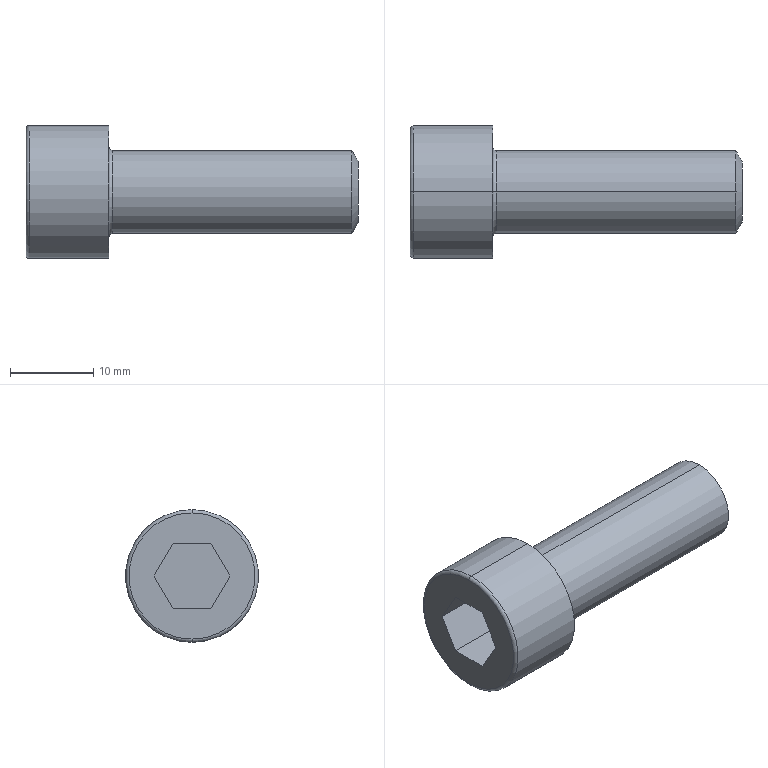Part | SolidWorks | features BaseBody 1 | 1 solid | 20 faces | box 40 x 16 x 16 mm | volume 4026 mm3 | plane 10 | torus 4 | cylinder 4 | cone 2 | commonest cylinder face diameters 10 x2 16 x2
STEP:
#1=CARTESIAN_POINT('',(40.,0.,3.701));
#2=VERTEX_POINT('',#1);
#3=CARTESIAN_POINT('',(40.,0.,-3.701));
#4=VERTEX_POINT('',#3);
#5=CARTESIAN_POINT('',(40.,0.,0.));
#6=DIRECTION('',(-1.,0.,0.));
#7=DIRECTION('',(0.,0.,1.));
#8=AXIS2_PLACEMENT_3D('',#5,#6,#7);
#9=CIRCLE('',#8,3.701);
#10=EDGE_CURVE('',#2,#4,#9,.T.);
#11=ORIENTED_EDGE('',*,*,#10,.T.);
#12=CARTESIAN_POINT('',(39.25,0.,-5.));
#13=VERTEX_POINT('',#12);
#14=CARTESIAN_POINT('',(39.25,0.,-5.));
#15=DIRECTION('',(-0.5,0.,-0.866));
#16=VECTOR('',#15,1000.);
#17=LINE('',#14,#16);
#18=EDGE_CURVE('',#4,#13,#17,.T.);
#19=ORIENTED_EDGE('',*,*,#18,.T.);
#20=CARTESIAN_POINT('',(39.25,0.,5.));
#21=VERTEX_POINT('',#20);
#22=CARTESIAN_POINT('',(39.25,0.,0.));
#23=DIRECTION('',(-1.,0.,0.));
#24=DIRECTION('',(0.,0.,1.));
#25=AXIS2_PLACEMENT_3D('',#22,#23,#24);
#26=CIRCLE('',#25,5.);
#27=EDGE_CURVE('',#21,#13,#26,.T.);
#28=ORIENTED_EDGE('',*,*,#27,.F.);
#29=CARTESIAN_POINT('',(39.25,0.,5.));
#30=DIRECTION('',(-0.5,0.,0.866));
#31=VECTOR('',#30,1000.);
#32=LINE('',#29,#31);
#33=EDGE_CURVE('',#2,#21,#32,.T.);
#34=ORIENTED_EDGE('',*,*,#33,.F.);
#35=EDGE_LOOP('',(#11,#19,#28,#34));
#36=FACE_OUTER_BOUND('',#35,.T.);
#37=CARTESIAN_POINT('',(39.25,0.,0.));
#38=DIRECTION('',(-1.,0.,0.));
#39=DIRECTION('',(0.,0.,1.));
#40=AXIS2_PLACEMENT_3D('',#37,#38,#39);
#41=CONICAL_SURFACE('',#40,5.,1.047);
#42=ADVANCED_FACE('',(#36),#41,.T.);
#43=CARTESIAN_POINT('',(0.4,0.,-8.));
#44=VERTEX_POINT('',#43);
#45=CARTESIAN_POINT('',(0.4,0.,8.));
#46=VERTEX_POINT('',#45);
#47=CARTESIAN_POINT('',(0.4,0.,0.));
#48=DIRECTION('',(1.,0.,0.));
#49=DIRECTION('',(0.,0.,1.));
#50=AXIS2_PLACEMENT_3D('',#47,#48,#49);
#51=CIRCLE('',#50,8.);
#52=EDGE_CURVE('',#44,#46,#51,.T.);
#53=ORIENTED_EDGE('',*,*,#52,.F.);
#54=CARTESIAN_POINT('',(0.,0.,-7.6));
#55=VERTEX_POINT('',#54);
#56=CARTESIAN_POINT('',(0.4,0.,-7.6));
#57=DIRECTION('',(0.,1.,0.));
#58=DIRECTION('',(0.,0.,1.));
#59=AXIS2_PLACEMENT_3D('',#56,#57,#58);
#60=CIRCLE('',#59,0.4);
#61=EDGE_CURVE('',#44,#55,#60,.T.);
#62=ORIENTED_EDGE('',*,*,#61,.T.);
#63=CARTESIAN_POINT('',(0.,0.,7.6));
#64=VERTEX_POINT('',#63);
#65=CARTESIAN_POINT('',(0.,0.,0.));
#66=DIRECTION('',(-1.,0.,0.));
#67=DIRECTION('',(0.,0.,1.));
#68=AXIS2_PLACEMENT_3D('',#65,#66,#67);
#69=CIRCLE('',#68,7.6);
#70=EDGE_CURVE('',#64,#55,#69,.T.);
#71=ORIENTED_EDGE('',*,*,#70,.F.);
#72=CARTESIAN_POINT('',(0.4,0.,7.6));
#73=DIRECTION('',(0.,-1.,0.));
#74=DIRECTION('',(0.,0.,-1.));
#75=AXIS2_PLACEMENT_3D('',#72,#73,#74);
#76=CIRCLE('',#75,0.4);
#77=EDGE_CURVE('',#46,#64,#76,.T.);
#78=ORIENTED_EDGE('',*,*,#77,.F.);
#79=EDGE_LOOP('',(#53,#62,#71,#78));
#80=FACE_OUTER_BOUND('',#79,.T.);
#81=CARTESIAN_POINT('',(0.4,0.,0.));
#82=DIRECTION('',(-1.,0.,0.));
#83=DIRECTION('',(0.,0.,1.));
#84=AXIS2_PLACEMENT_3D('',#81,#82,#83);
#85=TOROIDAL_SURFACE('',#84,7.6,0.4);
#86=ADVANCED_FACE('',(#80),#85,.T.);
#87=CARTESIAN_POINT('',(10.4,0.,5.));
#88=VERTEX_POINT('',#87);
#89=CARTESIAN_POINT('',(10.4,0.,-5.));
#90=VERTEX_POINT('',#89);
#91=CARTESIAN_POINT('',(10.4,0.,0.));
#92=DIRECTION('',(1.,0.,0.));
#93=DIRECTION('',(0.,0.,-1.));
#94=AXIS2_PLACEMENT_3D('',#91,#92,#93);
#95=CIRCLE('',#94,5.);
#96=EDGE_CURVE('',#88,#90,#95,.T.);
#97=ORIENTED_EDGE('',*,*,#96,.F.);
#98=CARTESIAN_POINT('',(10.,0.,5.4));
#99=VERTEX_POINT('',#98);
#100=CARTESIAN_POINT('',(10.4,0.,5.4));
#101=DIRECTION('',(0.,1.,0.));
#102=DIRECTION('',(0.,0.,1.));
#103=AXIS2_PLACEMENT_3D('',#100,#101,#102);
#104=CIRCLE('',#103,0.4);
#105=EDGE_CURVE('',#88,#99,#104,.T.);
#106=ORIENTED_EDGE('',*,*,#105,.T.);
#107=CARTESIAN_POINT('',(10.,0.,-5.4));
#108=VERTEX_POINT('',#107);
#109=CARTESIAN_POINT('',(10.,0.,0.));
#110=DIRECTION('',(1.,0.,0.));
#111=DIRECTION('',(0.,0.,-1.));
#112=AXIS2_PLACEMENT_3D('',#109,#110,#111);
#113=CIRCLE('',#112,5.4);
#114=EDGE_CURVE('',#99,#108,#113,.T.);
#115=ORIENTED_EDGE('',*,*,#114,.T.);
#116=CARTESIAN_POINT('',(10.4,0.,-5.4));
#117=DIRECTION('',(0.,-1.,0.));
#118=DIRECTION('',(0.,0.,-1.));
#119=AXIS2_PLACEMENT_3D('',#116,#117,#118);
#120=CIRCLE('',#119,0.4);
#121=EDGE_CURVE('',#90,#108,#120,.T.);
#122=ORIENTED_EDGE('',*,*,#121,.F.);
#123=EDGE_LOOP('',(#97,#106,#115,#122));
#124=FACE_OUTER_BOUND('',#123,.T.);
#125=CARTESIAN_POINT('',(10.4,0.,0.));
#126=DIRECTION('',(1.,0.,0.));
#127=DIRECTION('',(0.,0.,-1.));
#128=AXIS2_PLACEMENT_3D('',#125,#126,#127);
#129=TOROIDAL_SURFACE('',#128,5.4,0.4);
#130=ADVANCED_FACE('',(#124),#129,.F.);
#131=ORIENTED_EDGE('',*,*,#52,.T.);
#132=CARTESIAN_POINT('',(10.,0.,8.));
#133=VERTEX_POINT('',#132);
#134=CARTESIAN_POINT('',(0.,0.,8.));
#135=DIRECTION('',(1.,0.,0.));
#136=VECTOR('',#135,1000.);
#137=LINE('',#134,#136);
#138=EDGE_CURVE('',#46,#133,#137,.T.);
#139=ORIENTED_EDGE('',*,*,#138,.T.);
#140=CARTESIAN_POINT('',(10.,0.,-8.));
#141=VERTEX_POINT('',#140);
#142=CARTESIAN_POINT('',(10.,0.,0.));
#143=DIRECTION('',(1.,0.,0.));
#144=DIRECTION('',(0.,0.,-1.));
#145=AXIS2_PLACEMENT_3D('',#142,#143,#144);
#146=CIRCLE('',#145,8.);
#147=EDGE_CURVE('',#141,#133,#146,.T.);
#148=ORIENTED_EDGE('',*,*,#147,.F.);
#149=CARTESIAN_POINT('',(0.,0.,-8.));
#150=DIRECTION('',(1.,0.,0.));
#151=VECTOR('',#150,1000.);
#152=LINE('',#149,#151);
#153=EDGE_CURVE('',#44,#141,#152,.T.);
#154=ORIENTED_EDGE('',*,*,#153,.F.);
#155=EDGE_LOOP('',(#131,#139,#148,#154));
#156=FACE_OUTER_BOUND('',#155,.T.);
#157=CARTESIAN_POINT('',(0.,0.,0.));
#158=DIRECTION('',(1.,0.,0.));
#159=DIRECTION('',(0.,0.,-1.));
#160=AXIS2_PLACEMENT_3D('',#157,#158,#159);
#161=CYLINDRICAL_SURFACE('',#160,8.);
#162=ADVANCED_FACE('',(#156),#161,.T.);
#163=CARTESIAN_POINT('',(10.4,0.,0.));
#164=DIRECTION('',(1.,0.,0.));
#165=DIRECTION('',(0.,0.,-1.));
#166=AXIS2_PLACEMENT_3D('',#163,#164,#165);
#167=CIRCLE('',#166,5.);
#168=EDGE_CURVE('',#90,#88,#167,.T.);
#169=ORIENTED_EDGE('',*,*,#168,.T.);
#170=CARTESIAN_POINT('',(0.,0.,5.));
#171=DIRECTION('',(1.,0.,0.));
#172=VECTOR('',#171,1000.);
#173=LINE('',#170,#172);
#174=EDGE_CURVE('',#88,#21,#173,.T.);
#175=ORIENTED_EDGE('',*,*,#174,.T.);
#176=ORIENTED_EDGE('',*,*,#27,.T.);
#177=CARTESIAN_POINT('',(0.,0.,-5.));
#178=DIRECTION('',(1.,0.,0.));
#179=VECTOR('',#178,1000.);
#180=LINE('',#177,#179);
#181=EDGE_CURVE('',#90,#13,#180,.T.);
#182=ORIENTED_EDGE('',*,*,#181,.F.);
#183=EDGE_LOOP('',(#169,#175,#176,#182));
#184=FACE_OUTER_BOUND('',#183,.T.);
#185=CARTESIAN_POINT('',(0.,0.,0.));
#186=DIRECTION('',(1.,0.,0.));
#187=DIRECTION('',(0.,0.,-1.));
#188=AXIS2_PLACEMENT_3D('',#185,#186,#187);
#189=CYLINDRICAL_SURFACE('',#188,5.);
#190=ADVANCED_FACE('',(#184),#189,.T.);
#191=ORIENTED_EDGE('',*,*,#174,.F.);
#192=ORIENTED_EDGE('',*,*,#96,.T.);
#193=ORIENTED_EDGE('',*,*,#181,.T.);
#194=CARTESIAN_POINT('',(39.25,0.,0.));
#195=DIRECTION('',(-1.,0.,0.));
#196=DIRECTION('',(0.,0.,1.));
#197=AXIS2_PLACEMENT_3D('',#194,#195,#196);
#198=CIRCLE('',#197,5.);
#199=EDGE_CURVE('',#13,#21,#198,.T.);
#200=ORIENTED_EDGE('',*,*,#199,.T.);
#201=EDGE_LOOP('',(#191,#192,#193,#200));
#202=FACE_OUTER_BOUND('',#201,.T.);
#203=CARTESIAN_POINT('',(0.,0.,0.));
#204=DIRECTION('',(1.,0.,0.));
#205=DIRECTION('',(0.,0.,-1.));
#206=AXIS2_PLACEMENT_3D('',#203,#204,#205);
#207=CYLINDRICAL_SURFACE('',#206,5.);
#208=ADVANCED_FACE('',(#202),#207,.T.);
#209=ORIENTED_EDGE('',*,*,#70,.T.);
#210=CARTESIAN_POINT('',(0.,0.,0.));
#211=DIRECTION('',(-1.,0.,0.));
#212=DIRECTION('',(0.,0.,1.));
#213=AXIS2_PLACEMENT_3D('',#210,#211,#212);
#214=CIRCLE('',#213,7.6);
#215=EDGE_CURVE('',#55,#64,#214,.T.);
#216=ORIENTED_EDGE('',*,*,#215,.T.);
#217=EDGE_LOOP('',(#209,#216));
#218=FACE_OUTER_BOUND('',#217,.T.);
#219=CARTESIAN_POINT('',(0.,-4.575,0.));
#220=VERTEX_POINT('',#219);
#221=CARTESIAN_POINT('',(0.,-2.288,3.962));
#222=VERTEX_POINT('',#221);
#223=CARTESIAN_POINT('',(0.,-4.575,0.));
#224=DIRECTION('',(0.,0.5,0.866));
#225=VECTOR('',#224,1000.);
#226=LINE('',#223,#225);
#227=EDGE_CURVE('',#220,#222,#226,.T.);
#228=ORIENTED_EDGE('',*,*,#227,.F.);
#229=CARTESIAN_POINT('',(0.,-2.288,-3.962));
#230=VERTEX_POINT('',#229);
#231=CARTESIAN_POINT('',(0.,-2.288,-3.962));
#232=DIRECTION('',(0.,-0.5,0.866));
#233=VECTOR('',#232,1000.);
#234=LINE('',#231,#233);
#235=EDGE_CURVE('',#230,#220,#234,.T.);
#236=ORIENTED_EDGE('',*,*,#235,.F.);
#237=CARTESIAN_POINT('',(0.,2.288,-3.962));
#238=VERTEX_POINT('',#237);
#239=CARTESIAN_POINT('',(0.,2.288,-3.962));
#240=DIRECTION('',(0.,-1.,0.));
#241=VECTOR('',#240,1000.);
#242=LINE('',#239,#241);
#243=EDGE_CURVE('',#238,#230,#242,.T.);
#244=ORIENTED_EDGE('',*,*,#243,.F.);
#245=CARTESIAN_POINT('',(0.,4.575,0.));
#246=VERTEX_POINT('',#245);
#247=CARTESIAN_POINT('',(0.,4.575,0.));
#248=DIRECTION('',(0.,-0.5,-0.866));
#249=VECTOR('',#248,1000.);
#250=LINE('',#247,#249);
#251=EDGE_CURVE('',#246,#238,#250,.T.);
#252=ORIENTED_EDGE('',*,*,#251,.F.);
#253=CARTESIAN_POINT('',(0.,2.288,3.962));
#254=VERTEX_POINT('',#253);
#255=CARTESIAN_POINT('',(0.,2.288,3.962));
#256=DIRECTION('',(0.,0.5,-0.866));
#257=VECTOR('',#256,1000.);
#258=LINE('',#255,#257);
#259=EDGE_CURVE('',#254,#246,#258,.T.);
#260=ORIENTED_EDGE('',*,*,#259,.F.);
#261=CARTESIAN_POINT('',(0.,-2.288,3.962));
#262=DIRECTION('',(0.,1.,0.));
#263=VECTOR('',#262,1000.);
#264=LINE('',#261,#263);
#265=EDGE_CURVE('',#222,#254,#264,.T.);
#266=ORIENTED_EDGE('',*,*,#265,.F.);
#267=EDGE_LOOP('',(#228,#236,#244,#252,#260,#266));
#268=FACE_BOUND('',#267,.T.);
#269=CARTESIAN_POINT('',(0.,0.,0.));
#270=DIRECTION('',(-1.,0.,0.));
#271=DIRECTION('',(0.,0.,1.));
#272=AXIS2_PLACEMENT_3D('',#269,#270,#271);
#273=PLANE('',#272);
#274=ADVANCED_FACE('',(#218,#268),#273,.T.);
#275=ORIENTED_EDGE('',*,*,#138,.F.);
#276=CARTESIAN_POINT('',(0.4,0.,0.));
#277=DIRECTION('',(1.,0.,0.));
#278=DIRECTION('',(0.,0.,1.));
#279=AXIS2_PLACEMENT_3D('',#276,#277,#278);
#280=CIRCLE('',#279,8.);
#281=EDGE_CURVE('',#46,#44,#280,.T.);
#282=ORIENTED_EDGE('',*,*,#281,.T.);
#283=ORIENTED_EDGE('',*,*,#153,.T.);
#284=CARTESIAN_POINT('',(10.,0.,0.));
#285=DIRECTION('',(1.,0.,0.));
#286=DIRECTION('',(0.,0.,-1.));
#287=AXIS2_PLACEMENT_3D('',#284,#285,#286);
#288=CIRCLE('',#287,8.);
#289=EDGE_CURVE('',#133,#141,#288,.T.);
#290=ORIENTED_EDGE('',*,*,#289,.F.);
#291=EDGE_LOOP('',(#275,#282,#283,#290));
#292=FACE_OUTER_BOUND('',#291,.T.);
#293=CARTESIAN_POINT('',(0.,0.,0.));
#294=DIRECTION('',(1.,0.,0.));
#295=DIRECTION('',(0.,0.,-1.));
#296=AXIS2_PLACEMENT_3D('',#293,#294,#295);
#297=CYLINDRICAL_SURFACE('',#296,8.);
#298=ADVANCED_FACE('',(#292),#297,.T.);
#299=ORIENTED_EDGE('',*,*,#147,.T.);
#300=ORIENTED_EDGE('',*,*,#289,.T.);
#301=EDGE_LOOP('',(#299,#300));
#302=FACE_OUTER_BOUND('',#301,.T.);
#303=CARTESIAN_POINT('',(10.,0.,0.));
#304=DIRECTION('',(1.,0.,0.));
#305=DIRECTION('',(0.,0.,-1.));
#306=AXIS2_PLACEMENT_3D('',#303,#304,#305);
#307=CIRCLE('',#306,5.4);
#308=EDGE_CURVE('',#108,#99,#307,.T.);
#309=ORIENTED_EDGE('',*,*,#308,.F.);
#310=ORIENTED_EDGE('',*,*,#114,.F.);
#311=EDGE_LOOP('',(#309,#310));
#312=FACE_BOUND('',#311,.T.);
#313=CARTESIAN_POINT('',(10.,8.,0.));
#314=DIRECTION('',(1.,0.,0.));
#315=DIRECTION('',(0.,0.,-1.));
#316=AXIS2_PLACEMENT_3D('',#313,#314,#315);
#317=PLANE('',#316);
#318=ADVANCED_FACE('',(#302,#312),#317,.T.);
#319=ORIENTED_EDGE('',*,*,#105,.F.);
#320=ORIENTED_EDGE('',*,*,#168,.F.);
#321=ORIENTED_EDGE('',*,*,#121,.T.);
#322=ORIENTED_EDGE('',*,*,#308,.T.);
#323=EDGE_LOOP('',(#319,#320,#321,#322));
#324=FACE_OUTER_BOUND('',#323,.T.);
#325=CARTESIAN_POINT('',(10.4,0.,0.));
#326=DIRECTION('',(1.,0.,0.));
#327=DIRECTION('',(0.,0.,-1.));
#328=AXIS2_PLACEMENT_3D('',#325,#326,#327);
#329=TOROIDAL_SURFACE('',#328,5.4,0.4);
#330=ADVANCED_FACE('',(#324),#329,.F.);
#331=ORIENTED_EDGE('',*,*,#227,.T.);
#332=CARTESIAN_POINT('',(6.,-2.288,3.962));
#333=VERTEX_POINT('',#332);
#334=CARTESIAN_POINT('',(6.,-2.288,3.962));
#335=DIRECTION('',(-1.,0.,0.));
#336=VECTOR('',#335,1000.);
#337=LINE('',#334,#336);
#338=EDGE_CURVE('',#333,#222,#337,.T.);
#339=ORIENTED_EDGE('',*,*,#338,.F.);
#340=CARTESIAN_POINT('',(6.,-4.575,0.));
#341=VERTEX_POINT('',#340);
#342=CARTESIAN_POINT('',(6.,-4.575,0.));
#343=DIRECTION('',(0.,0.5,0.866));
#344=VECTOR('',#343,1000.);
#345=LINE('',#342,#344);
#346=EDGE_CURVE('',#341,#333,#345,.T.);
#347=ORIENTED_EDGE('',*,*,#346,.F.);
#348=CARTESIAN_POINT('',(6.,-4.575,0.));
#349=DIRECTION('',(-1.,0.,0.));
#350=VECTOR('',#349,1000.);
#351=LINE('',#348,#350);
#352=EDGE_CURVE('',#341,#220,#351,.T.);
#353=ORIENTED_EDGE('',*,*,#352,.T.);
#354=EDGE_LOOP('',(#331,#339,#347,#353));
#355=FACE_OUTER_BOUND('',#354,.T.);
#356=CARTESIAN_POINT('',(6.,-4.575,0.));
#357=DIRECTION('',(0.,-0.866,0.5));
#358=DIRECTION('',(0.,-0.5,-0.866));
#359=AXIS2_PLACEMENT_3D('',#356,#357,#358);
#360=PLANE('',#359);
#361=ADVANCED_FACE('',(#355),#360,.F.);
#362=ORIENTED_EDGE('',*,*,#235,.T.);
#363=ORIENTED_EDGE('',*,*,#352,.F.);
#364=CARTESIAN_POINT('',(6.,-2.288,-3.962));
#365=VERTEX_POINT('',#364);
#366=CARTESIAN_POINT('',(6.,-2.288,-3.962));
#367=DIRECTION('',(0.,-0.5,0.866));
#368=VECTOR('',#367,1000.);
#369=LINE('',#366,#368);
#370=EDGE_CURVE('',#365,#341,#369,.T.);
#371=ORIENTED_EDGE('',*,*,#370,.F.);
#372=CARTESIAN_POINT('',(6.,-2.288,-3.962));
#373=DIRECTION('',(-1.,0.,0.));
#374=VECTOR('',#373,1000.);
#375=LINE('',#372,#374);
#376=EDGE_CURVE('',#365,#230,#375,.T.);
#377=ORIENTED_EDGE('',*,*,#376,.T.);
#378=EDGE_LOOP('',(#362,#363,#371,#377));
#379=FACE_OUTER_BOUND('',#378,.T.);
#380=CARTESIAN_POINT('',(6.,-2.288,-3.962));
#381=DIRECTION('',(0.,-0.866,-0.5));
#382=DIRECTION('',(0.,0.5,-0.866));
#383=AXIS2_PLACEMENT_3D('',#380,#381,#382);
#384=PLANE('',#383);
#385=ADVANCED_FACE('',(#379),#384,.F.);
#386=ORIENTED_EDGE('',*,*,#243,.T.);
#387=ORIENTED_EDGE('',*,*,#376,.F.);
#388=CARTESIAN_POINT('',(6.,2.288,-3.962));
#389=VERTEX_POINT('',#388);
#390=CARTESIAN_POINT('',(6.,2.288,-3.962));
#391=DIRECTION('',(0.,-1.,0.));
#392=VECTOR('',#391,1000.);
#393=LINE('',#390,#392);
#394=EDGE_CURVE('',#389,#365,#393,.T.);
#395=ORIENTED_EDGE('',*,*,#394,.F.);
#396=CARTESIAN_POINT('',(6.,2.288,-3.962));
#397=DIRECTION('',(-1.,0.,0.));
#398=VECTOR('',#397,1000.);
#399=LINE('',#396,#398);
#400=EDGE_CURVE('',#389,#238,#399,.T.);
#401=ORIENTED_EDGE('',*,*,#400,.T.);
#402=EDGE_LOOP('',(#386,#387,#395,#401));
#403=FACE_OUTER_BOUND('',#402,.T.);
#404=CARTESIAN_POINT('',(6.,2.288,-3.962));
#405=DIRECTION('',(0.,0.,-1.));
#406=DIRECTION('',(0.,1.,0.));
#407=AXIS2_PLACEMENT_3D('',#404,#405,#406);
#408=PLANE('',#407);
#409=ADVANCED_FACE('',(#403),#408,.F.);
#410=ORIENTED_EDGE('',*,*,#251,.T.);
#411=ORIENTED_EDGE('',*,*,#400,.F.);
#412=CARTESIAN_POINT('',(6.,4.575,0.));
#413=VERTEX_POINT('',#412);
#414=CARTESIAN_POINT('',(6.,4.575,0.));
#415=DIRECTION('',(0.,-0.5,-0.866));
#416=VECTOR('',#415,1000.);
#417=LINE('',#414,#416);
#418=EDGE_CURVE('',#413,#389,#417,.T.);
#419=ORIENTED_EDGE('',*,*,#418,.F.);
#420=CARTESIAN_POINT('',(6.,4.575,0.));
#421=DIRECTION('',(-1.,0.,0.));
#422=VECTOR('',#421,1000.);
#423=LINE('',#420,#422);
#424=EDGE_CURVE('',#413,#246,#423,.T.);
#425=ORIENTED_EDGE('',*,*,#424,.T.);
#426=EDGE_LOOP('',(#410,#411,#419,#425));
#427=FACE_OUTER_BOUND('',#426,.T.);
#428=CARTESIAN_POINT('',(6.,4.575,0.));
#429=DIRECTION('',(0.,0.866,-0.5));
#430=DIRECTION('',(0.,0.5,0.866));
#431=AXIS2_PLACEMENT_3D('',#428,#429,#430);
#432=PLANE('',#431);
#433=ADVANCED_FACE('',(#427),#432,.F.);
#434=ORIENTED_EDGE('',*,*,#259,.T.);
#435=ORIENTED_EDGE('',*,*,#424,.F.);
#436=CARTESIAN_POINT('',(6.,2.288,3.962));
#437=VERTEX_POINT('',#436);
#438=CARTESIAN_POINT('',(6.,2.288,3.962));
#439=DIRECTION('',(0.,0.5,-0.866));
#440=VECTOR('',#439,1000.);
#441=LINE('',#438,#440);
#442=EDGE_CURVE('',#437,#413,#441,.T.);
#443=ORIENTED_EDGE('',*,*,#442,.F.);
#444=CARTESIAN_POINT('',(6.,2.288,3.962));
#445=DIRECTION('',(-1.,0.,0.));
#446=VECTOR('',#445,1000.);
#447=LINE('',#444,#446);
#448=EDGE_CURVE('',#437,#254,#447,.T.);
#449=ORIENTED_EDGE('',*,*,#448,.T.);
#450=EDGE_LOOP('',(#434,#435,#443,#449));
#451=FACE_OUTER_BOUND('',#450,.T.);
#452=CARTESIAN_POINT('',(6.,2.288,3.962));
#453=DIRECTION('',(0.,0.866,0.5));
#454=DIRECTION('',(0.,-0.5,0.866));
#455=AXIS2_PLACEMENT_3D('',#452,#453,#454);
#456=PLANE('',#455);
#457=ADVANCED_FACE('',(#451),#456,.F.);
#458=ORIENTED_EDGE('',*,*,#265,.T.);
#459=ORIENTED_EDGE('',*,*,#448,.F.);
#460=CARTESIAN_POINT('',(6.,-2.288,3.962));
#461=DIRECTION('',(0.,1.,0.));
#462=VECTOR('',#461,1000.);
#463=LINE('',#460,#462);
#464=EDGE_CURVE('',#333,#437,#463,.T.);
#465=ORIENTED_EDGE('',*,*,#464,.F.);
#466=ORIENTED_EDGE('',*,*,#338,.T.);
#467=EDGE_LOOP('',(#458,#459,#465,#466));
#468=FACE_OUTER_BOUND('',#467,.T.);
#469=CARTESIAN_POINT('',(6.,-2.288,3.962));
#470=DIRECTION('',(0.,0.,1.));
#471=DIRECTION('',(0.,-1.,0.));
#472=AXIS2_PLACEMENT_3D('',#469,#470,#471);
#473=PLANE('',#472);
#474=ADVANCED_FACE('',(#468),#473,.F.);
#475=ORIENTED_EDGE('',*,*,#346,.T.);
#476=ORIENTED_EDGE('',*,*,#464,.T.);
#477=ORIENTED_EDGE('',*,*,#442,.T.);
#478=ORIENTED_EDGE('',*,*,#418,.T.);
#479=ORIENTED_EDGE('',*,*,#394,.T.);
#480=ORIENTED_EDGE('',*,*,#370,.T.);
#481=EDGE_LOOP('',(#475,#476,#477,#478,#479,#480));
#482=FACE_OUTER_BOUND('',#481,.T.);
#483=CARTESIAN_POINT('',(6.,-2.288,3.962));
#484=DIRECTION('',(-1.,0.,0.));
#485=DIRECTION('',(0.,0.,1.));
#486=AXIS2_PLACEMENT_3D('',#483,#484,#485);
#487=PLANE('',#486);
#488=ADVANCED_FACE('',(#482),#487,.T.);
#489=ORIENTED_EDGE('',*,*,#61,.F.);
#490=ORIENTED_EDGE('',*,*,#281,.F.);
#491=ORIENTED_EDGE('',*,*,#77,.T.);
#492=ORIENTED_EDGE('',*,*,#215,.F.);
#493=EDGE_LOOP('',(#489,#490,#491,#492));
#494=FACE_OUTER_BOUND('',#493,.T.);
#495=CARTESIAN_POINT('',(0.4,0.,0.));
#496=DIRECTION('',(-1.,0.,0.));
#497=DIRECTION('',(0.,0.,1.));
#498=AXIS2_PLACEMENT_3D('',#495,#496,#497);
#499=TOROIDAL_SURFACE('',#498,7.6,0.4);
#500=ADVANCED_FACE('',(#494),#499,.T.);
#501=ORIENTED_EDGE('',*,*,#18,.F.);
#502=CARTESIAN_POINT('',(40.,0.,0.));
#503=DIRECTION('',(-1.,0.,0.));
#504=DIRECTION('',(0.,0.,1.));
#505=AXIS2_PLACEMENT_3D('',#502,#503,#504);
#506=CIRCLE('',#505,3.701);
#507=EDGE_CURVE('',#4,#2,#506,.T.);
#508=ORIENTED_EDGE('',*,*,#507,.T.);
#509=ORIENTED_EDGE('',*,*,#33,.T.);
#510=ORIENTED_EDGE('',*,*,#199,.F.);
#511=EDGE_LOOP('',(#501,#508,#509,#510));
#512=FACE_OUTER_BOUND('',#511,.T.);
#513=CARTESIAN_POINT('',(39.25,0.,0.));
#514=DIRECTION('',(-1.,0.,0.));
#515=DIRECTION('',(0.,0.,1.));
#516=AXIS2_PLACEMENT_3D('',#513,#514,#515);
#517=CONICAL_SURFACE('',#516,5.,1.047);
#518=ADVANCED_FACE('',(#512),#517,.T.);
#519=ORIENTED_EDGE('',*,*,#10,.F.);
#520=ORIENTED_EDGE('',*,*,#507,.F.);
#521=EDGE_LOOP('',(#519,#520));
#522=FACE_OUTER_BOUND('',#521,.T.);
#523=CARTESIAN_POINT('',(40.,5.,0.));
#524=DIRECTION('',(1.,0.,0.));
#525=DIRECTION('',(0.,0.,-1.));
#526=AXIS2_PLACEMENT_3D('',#523,#524,#525);
#527=PLANE('',#526);
#528=ADVANCED_FACE('',(#522),#527,.T.);
#529=CLOSED_SHELL('',(#42,#86,#130,#162,#190,#208,#274,#298,#318,#330,#361,#385,#409,#433,#457,#474,#488,#500,#518,#528));
#530=MANIFOLD_SOLID_BREP('',#529);
#531=CARTESIAN_POINT('',(0.,0.,0.));
#532=DIRECTION('',(0.,0.,1.));
#533=DIRECTION('',(1.,0.,0.));
#534=AXIS2_PLACEMENT_3D('',#531,#532,#533);
#535=(LENGTH_UNIT()NAMED_UNIT(*)SI_UNIT(.MILLI.,.METRE.));
#536=UNCERTAINTY_MEASURE_WITH_UNIT(LENGTH_MEASURE(0.00001),#535,'','');
#537=(NAMED_UNIT(*)PLANE_ANGLE_UNIT()SI_UNIT($,.RADIAN.));
#538=(NAMED_UNIT(*)SI_UNIT($,.STERADIAN.)SOLID_ANGLE_UNIT());
#539=(GEOMETRIC_REPRESENTATION_CONTEXT(3)GLOBAL_UNCERTAINTY_ASSIGNED_CONTEXT((#536))GLOBAL_UNIT_ASSIGNED_CONTEXT((#535,#537,#538))REPRESENTATION_CONTEXT('',''));
#540=ADVANCED_BREP_SHAPE_REPRESENTATION('',(#530,#534),#539);